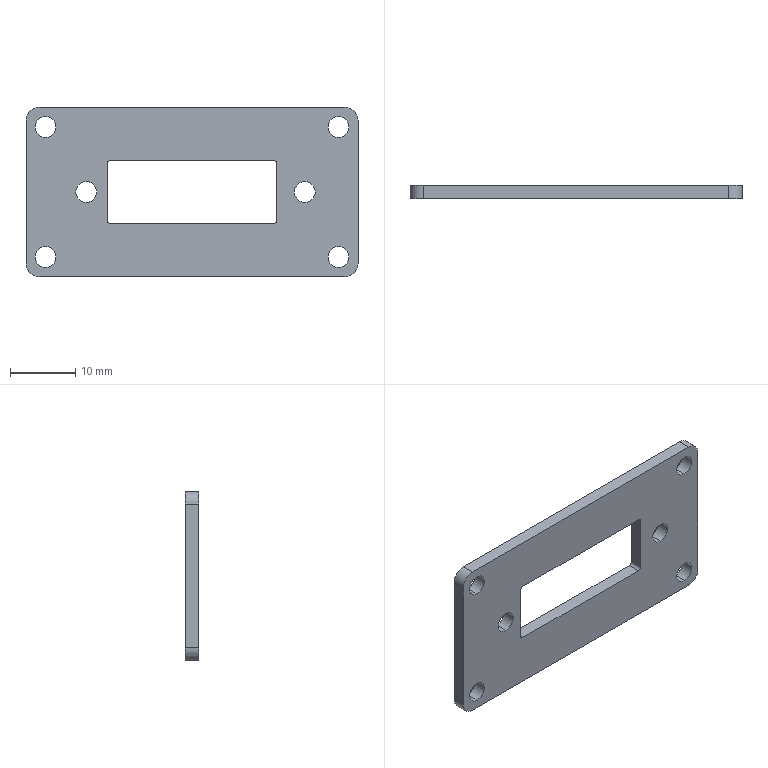Part | SolidWorks | features Cut 1, Extrusion 1, Fillet 1 | 1 solid | 30 faces | box 51 x 2 x 26 mm | volume 2048 mm3 | cylinder 20 | plane 10 | commonest cylinder face diameters 3.2 x12 1 x4 4 x4
STEP:
#1=CARTESIAN_POINT('',(17.311,2.,1.6));
#2=VERTEX_POINT('',#1);
#3=CARTESIAN_POINT('',(17.311,2.,-1.6));
#4=VERTEX_POINT('',#3);
#5=CARTESIAN_POINT('',(17.311,2.,0.));
#6=DIRECTION('',(0.,-1.,0.));
#7=DIRECTION('',(0.,0.,-1.));
#8=AXIS2_PLACEMENT_3D('',#5,#6,#7);
#9=CIRCLE('',#8,1.6);
#10=EDGE_CURVE('',#2,#4,#9,.T.);
#11=ORIENTED_EDGE('',*,*,#10,.F.);
#12=CARTESIAN_POINT('',(17.311,0.,1.6));
#13=VERTEX_POINT('',#12);
#14=CARTESIAN_POINT('',(17.311,2.,1.6));
#15=DIRECTION('',(0.,-1.,0.));
#16=VECTOR('',#15,1000.);
#17=LINE('',#14,#16);
#18=EDGE_CURVE('',#2,#13,#17,.T.);
#19=ORIENTED_EDGE('',*,*,#18,.T.);
#20=CARTESIAN_POINT('',(17.311,0.,-1.6));
#21=VERTEX_POINT('',#20);
#22=CARTESIAN_POINT('',(17.311,0.,0.));
#23=DIRECTION('',(0.,-1.,0.));
#24=DIRECTION('',(0.,0.,-1.));
#25=AXIS2_PLACEMENT_3D('',#22,#23,#24);
#26=CIRCLE('',#25,1.6);
#27=EDGE_CURVE('',#13,#21,#26,.T.);
#28=ORIENTED_EDGE('',*,*,#27,.T.);
#29=CARTESIAN_POINT('',(17.311,2.,-1.6));
#30=DIRECTION('',(0.,-1.,0.));
#31=VECTOR('',#30,1000.);
#32=LINE('',#29,#31);
#33=EDGE_CURVE('',#4,#21,#32,.T.);
#34=ORIENTED_EDGE('',*,*,#33,.F.);
#35=EDGE_LOOP('',(#11,#19,#28,#34));
#36=FACE_OUTER_BOUND('',#35,.T.);
#37=CARTESIAN_POINT('',(17.311,2.,0.));
#38=DIRECTION('',(0.,-1.,0.));
#39=DIRECTION('',(0.,0.,-1.));
#40=AXIS2_PLACEMENT_3D('',#37,#38,#39);
#41=CYLINDRICAL_SURFACE('',#40,1.6);
#42=ADVANCED_FACE('',(#36),#41,.F.);
#43=CARTESIAN_POINT('',(-16.25,2.,1.6));
#44=VERTEX_POINT('',#43);
#45=CARTESIAN_POINT('',(-16.25,2.,-1.6));
#46=VERTEX_POINT('',#45);
#47=CARTESIAN_POINT('',(-16.25,2.,0.));
#48=DIRECTION('',(0.,-1.,0.));
#49=DIRECTION('',(0.,0.,-1.));
#50=AXIS2_PLACEMENT_3D('',#47,#48,#49);
#51=CIRCLE('',#50,1.6);
#52=EDGE_CURVE('',#44,#46,#51,.T.);
#53=ORIENTED_EDGE('',*,*,#52,.F.);
#54=CARTESIAN_POINT('',(-16.25,0.,1.6));
#55=VERTEX_POINT('',#54);
#56=CARTESIAN_POINT('',(-16.25,2.,1.6));
#57=DIRECTION('',(0.,-1.,0.));
#58=VECTOR('',#57,1000.);
#59=LINE('',#56,#58);
#60=EDGE_CURVE('',#44,#55,#59,.T.);
#61=ORIENTED_EDGE('',*,*,#60,.T.);
#62=CARTESIAN_POINT('',(-16.25,0.,-1.6));
#63=VERTEX_POINT('',#62);
#64=CARTESIAN_POINT('',(-16.25,0.,0.));
#65=DIRECTION('',(0.,-1.,0.));
#66=DIRECTION('',(0.,0.,-1.));
#67=AXIS2_PLACEMENT_3D('',#64,#65,#66);
#68=CIRCLE('',#67,1.6);
#69=EDGE_CURVE('',#55,#63,#68,.T.);
#70=ORIENTED_EDGE('',*,*,#69,.T.);
#71=CARTESIAN_POINT('',(-16.25,2.,-1.6));
#72=DIRECTION('',(0.,-1.,0.));
#73=VECTOR('',#72,1000.);
#74=LINE('',#71,#73);
#75=EDGE_CURVE('',#46,#63,#74,.T.);
#76=ORIENTED_EDGE('',*,*,#75,.F.);
#77=EDGE_LOOP('',(#53,#61,#70,#76));
#78=FACE_OUTER_BOUND('',#77,.T.);
#79=CARTESIAN_POINT('',(-16.25,2.,0.));
#80=DIRECTION('',(0.,-1.,0.));
#81=DIRECTION('',(0.,0.,-1.));
#82=AXIS2_PLACEMENT_3D('',#79,#80,#81);
#83=CYLINDRICAL_SURFACE('',#82,1.6);
#84=ADVANCED_FACE('',(#78),#83,.F.);
#85=CARTESIAN_POINT('',(-22.5,2.,8.4));
#86=VERTEX_POINT('',#85);
#87=CARTESIAN_POINT('',(-22.5,2.,11.6));
#88=VERTEX_POINT('',#87);
#89=CARTESIAN_POINT('',(-22.5,2.,10.));
#90=DIRECTION('',(0.,1.,0.));
#91=DIRECTION('',(0.,0.,1.));
#92=AXIS2_PLACEMENT_3D('',#89,#90,#91);
#93=CIRCLE('',#92,1.6);
#94=EDGE_CURVE('',#86,#88,#93,.T.);
#95=ORIENTED_EDGE('',*,*,#94,.T.);
#96=CARTESIAN_POINT('',(-22.5,0.,11.6));
#97=VERTEX_POINT('',#96);
#98=CARTESIAN_POINT('',(-22.5,2.,11.6));
#99=DIRECTION('',(0.,-1.,0.));
#100=VECTOR('',#99,1000.);
#101=LINE('',#98,#100);
#102=EDGE_CURVE('',#88,#97,#101,.T.);
#103=ORIENTED_EDGE('',*,*,#102,.T.);
#104=CARTESIAN_POINT('',(-22.5,0.,8.4));
#105=VERTEX_POINT('',#104);
#106=CARTESIAN_POINT('',(-22.5,0.,10.));
#107=DIRECTION('',(0.,1.,0.));
#108=DIRECTION('',(0.,0.,1.));
#109=AXIS2_PLACEMENT_3D('',#106,#107,#108);
#110=CIRCLE('',#109,1.6);
#111=EDGE_CURVE('',#105,#97,#110,.T.);
#112=ORIENTED_EDGE('',*,*,#111,.F.);
#113=CARTESIAN_POINT('',(-22.5,2.,8.4));
#114=DIRECTION('',(0.,-1.,0.));
#115=VECTOR('',#114,1000.);
#116=LINE('',#113,#115);
#117=EDGE_CURVE('',#86,#105,#116,.T.);
#118=ORIENTED_EDGE('',*,*,#117,.F.);
#119=EDGE_LOOP('',(#95,#103,#112,#118));
#120=FACE_OUTER_BOUND('',#119,.T.);
#121=CARTESIAN_POINT('',(-22.5,2.,10.));
#122=DIRECTION('',(0.,-1.,0.));
#123=DIRECTION('',(0.,0.,-1.));
#124=AXIS2_PLACEMENT_3D('',#121,#122,#123);
#125=CYLINDRICAL_SURFACE('',#124,1.6);
#126=ADVANCED_FACE('',(#120),#125,.F.);
#127=CARTESIAN_POINT('',(22.5,2.,8.4));
#128=VERTEX_POINT('',#127);
#129=CARTESIAN_POINT('',(22.5,2.,11.6));
#130=VERTEX_POINT('',#129);
#131=CARTESIAN_POINT('',(22.5,2.,10.));
#132=DIRECTION('',(0.,1.,0.));
#133=DIRECTION('',(0.,0.,1.));
#134=AXIS2_PLACEMENT_3D('',#131,#132,#133);
#135=CIRCLE('',#134,1.6);
#136=EDGE_CURVE('',#128,#130,#135,.T.);
#137=ORIENTED_EDGE('',*,*,#136,.T.);
#138=CARTESIAN_POINT('',(22.5,0.,11.6));
#139=VERTEX_POINT('',#138);
#140=CARTESIAN_POINT('',(22.5,2.,11.6));
#141=DIRECTION('',(0.,-1.,0.));
#142=VECTOR('',#141,1000.);
#143=LINE('',#140,#142);
#144=EDGE_CURVE('',#130,#139,#143,.T.);
#145=ORIENTED_EDGE('',*,*,#144,.T.);
#146=CARTESIAN_POINT('',(22.5,0.,8.4));
#147=VERTEX_POINT('',#146);
#148=CARTESIAN_POINT('',(22.5,0.,10.));
#149=DIRECTION('',(0.,1.,0.));
#150=DIRECTION('',(0.,0.,1.));
#151=AXIS2_PLACEMENT_3D('',#148,#149,#150);
#152=CIRCLE('',#151,1.6);
#153=EDGE_CURVE('',#147,#139,#152,.T.);
#154=ORIENTED_EDGE('',*,*,#153,.F.);
#155=CARTESIAN_POINT('',(22.5,2.,8.4));
#156=DIRECTION('',(0.,-1.,0.));
#157=VECTOR('',#156,1000.);
#158=LINE('',#155,#157);
#159=EDGE_CURVE('',#128,#147,#158,.T.);
#160=ORIENTED_EDGE('',*,*,#159,.F.);
#161=EDGE_LOOP('',(#137,#145,#154,#160));
#162=FACE_OUTER_BOUND('',#161,.T.);
#163=CARTESIAN_POINT('',(22.5,2.,10.));
#164=DIRECTION('',(0.,-1.,0.));
#165=DIRECTION('',(0.,0.,-1.));
#166=AXIS2_PLACEMENT_3D('',#163,#164,#165);
#167=CYLINDRICAL_SURFACE('',#166,1.6);
#168=ADVANCED_FACE('',(#162),#167,.F.);
#169=CARTESIAN_POINT('',(22.5,2.,-11.6));
#170=VERTEX_POINT('',#169);
#171=CARTESIAN_POINT('',(22.5,2.,-8.4));
#172=VERTEX_POINT('',#171);
#173=CARTESIAN_POINT('',(22.5,2.,-10.));
#174=DIRECTION('',(0.,1.,0.));
#175=DIRECTION('',(0.,0.,1.));
#176=AXIS2_PLACEMENT_3D('',#173,#174,#175);
#177=CIRCLE('',#176,1.6);
#178=EDGE_CURVE('',#170,#172,#177,.T.);
#179=ORIENTED_EDGE('',*,*,#178,.T.);
#180=CARTESIAN_POINT('',(22.5,0.,-8.4));
#181=VERTEX_POINT('',#180);
#182=CARTESIAN_POINT('',(22.5,2.,-8.4));
#183=DIRECTION('',(0.,-1.,0.));
#184=VECTOR('',#183,1000.);
#185=LINE('',#182,#184);
#186=EDGE_CURVE('',#172,#181,#185,.T.);
#187=ORIENTED_EDGE('',*,*,#186,.T.);
#188=CARTESIAN_POINT('',(22.5,0.,-11.6));
#189=VERTEX_POINT('',#188);
#190=CARTESIAN_POINT('',(22.5,0.,-10.));
#191=DIRECTION('',(0.,1.,0.));
#192=DIRECTION('',(0.,0.,1.));
#193=AXIS2_PLACEMENT_3D('',#190,#191,#192);
#194=CIRCLE('',#193,1.6);
#195=EDGE_CURVE('',#189,#181,#194,.T.);
#196=ORIENTED_EDGE('',*,*,#195,.F.);
#197=CARTESIAN_POINT('',(22.5,2.,-11.6));
#198=DIRECTION('',(0.,-1.,0.));
#199=VECTOR('',#198,1000.);
#200=LINE('',#197,#199);
#201=EDGE_CURVE('',#170,#189,#200,.T.);
#202=ORIENTED_EDGE('',*,*,#201,.F.);
#203=EDGE_LOOP('',(#179,#187,#196,#202));
#204=FACE_OUTER_BOUND('',#203,.T.);
#205=CARTESIAN_POINT('',(22.5,2.,-10.));
#206=DIRECTION('',(0.,-1.,0.));
#207=DIRECTION('',(0.,0.,-1.));
#208=AXIS2_PLACEMENT_3D('',#205,#206,#207);
#209=CYLINDRICAL_SURFACE('',#208,1.6);
#210=ADVANCED_FACE('',(#204),#209,.F.);
#211=CARTESIAN_POINT('',(-22.5,2.,-11.6));
#212=VERTEX_POINT('',#211);
#213=CARTESIAN_POINT('',(-22.5,2.,-8.4));
#214=VERTEX_POINT('',#213);
#215=CARTESIAN_POINT('',(-22.5,2.,-10.));
#216=DIRECTION('',(0.,1.,0.));
#217=DIRECTION('',(0.,0.,1.));
#218=AXIS2_PLACEMENT_3D('',#215,#216,#217);
#219=CIRCLE('',#218,1.6);
#220=EDGE_CURVE('',#212,#214,#219,.T.);
#221=ORIENTED_EDGE('',*,*,#220,.T.);
#222=CARTESIAN_POINT('',(-22.5,0.,-8.4));
#223=VERTEX_POINT('',#222);
#224=CARTESIAN_POINT('',(-22.5,2.,-8.4));
#225=DIRECTION('',(0.,-1.,0.));
#226=VECTOR('',#225,1000.);
#227=LINE('',#224,#226);
#228=EDGE_CURVE('',#214,#223,#227,.T.);
#229=ORIENTED_EDGE('',*,*,#228,.T.);
#230=CARTESIAN_POINT('',(-22.5,0.,-11.6));
#231=VERTEX_POINT('',#230);
#232=CARTESIAN_POINT('',(-22.5,0.,-10.));
#233=DIRECTION('',(0.,1.,0.));
#234=DIRECTION('',(0.,0.,1.));
#235=AXIS2_PLACEMENT_3D('',#232,#233,#234);
#236=CIRCLE('',#235,1.6);
#237=EDGE_CURVE('',#231,#223,#236,.T.);
#238=ORIENTED_EDGE('',*,*,#237,.F.);
#239=CARTESIAN_POINT('',(-22.5,2.,-11.6));
#240=DIRECTION('',(0.,-1.,0.));
#241=VECTOR('',#240,1000.);
#242=LINE('',#239,#241);
#243=EDGE_CURVE('',#212,#231,#242,.T.);
#244=ORIENTED_EDGE('',*,*,#243,.F.);
#245=EDGE_LOOP('',(#221,#229,#238,#244));
#246=FACE_OUTER_BOUND('',#245,.T.);
#247=CARTESIAN_POINT('',(-22.5,2.,-10.));
#248=DIRECTION('',(0.,-1.,0.));
#249=DIRECTION('',(0.,0.,-1.));
#250=AXIS2_PLACEMENT_3D('',#247,#248,#249);
#251=CYLINDRICAL_SURFACE('',#250,1.6);
#252=ADVANCED_FACE('',(#246),#251,.F.);
#253=CARTESIAN_POINT('',(17.311,2.,0.));
#254=DIRECTION('',(0.,-1.,0.));
#255=DIRECTION('',(0.,0.,-1.));
#256=AXIS2_PLACEMENT_3D('',#253,#254,#255);
#257=CIRCLE('',#256,1.6);
#258=EDGE_CURVE('',#4,#2,#257,.T.);
#259=ORIENTED_EDGE('',*,*,#258,.T.);
#260=ORIENTED_EDGE('',*,*,#10,.T.);
#261=EDGE_LOOP('',(#259,#260));
#262=FACE_BOUND('',#261,.T.);
#263=CARTESIAN_POINT('',(-16.25,2.,0.));
#264=DIRECTION('',(0.,-1.,0.));
#265=DIRECTION('',(0.,0.,-1.));
#266=AXIS2_PLACEMENT_3D('',#263,#264,#265);
#267=CIRCLE('',#266,1.6);
#268=EDGE_CURVE('',#46,#44,#267,.T.);
#269=ORIENTED_EDGE('',*,*,#268,.T.);
#270=ORIENTED_EDGE('',*,*,#52,.T.);
#271=EDGE_LOOP('',(#269,#270));
#272=FACE_BOUND('',#271,.T.);
#273=CARTESIAN_POINT('',(-13.05,2.,4.3));
#274=VERTEX_POINT('',#273);
#275=CARTESIAN_POINT('',(-13.05,2.,-4.3));
#276=VERTEX_POINT('',#275);
#277=CARTESIAN_POINT('',(-13.05,2.,-4.8));
#278=DIRECTION('',(0.,0.,-1.));
#279=VECTOR('',#278,1000.);
#280=LINE('',#277,#279);
#281=EDGE_CURVE('',#274,#276,#280,.T.);
#282=ORIENTED_EDGE('',*,*,#281,.T.);
#283=CARTESIAN_POINT('',(-12.55,2.,-4.8));
#284=VERTEX_POINT('',#283);
#285=CARTESIAN_POINT('',(-12.55,2.,-4.3));
#286=DIRECTION('',(0.,-1.,0.));
#287=DIRECTION('',(0.,0.,-1.));
#288=AXIS2_PLACEMENT_3D('',#285,#286,#287);
#289=CIRCLE('',#288,0.5);
#290=EDGE_CURVE('',#276,#284,#289,.T.);
#291=ORIENTED_EDGE('',*,*,#290,.T.);
#292=CARTESIAN_POINT('',(12.55,2.,-4.8));
#293=VERTEX_POINT('',#292);
#294=CARTESIAN_POINT('',(-13.05,2.,-4.8));
#295=DIRECTION('',(1.,0.,0.));
#296=VECTOR('',#295,1000.);
#297=LINE('',#294,#296);
#298=EDGE_CURVE('',#284,#293,#297,.T.);
#299=ORIENTED_EDGE('',*,*,#298,.T.);
#300=CARTESIAN_POINT('',(13.05,2.,-4.3));
#301=VERTEX_POINT('',#300);
#302=CARTESIAN_POINT('',(12.55,2.,-4.3));
#303=DIRECTION('',(0.,-1.,0.));
#304=DIRECTION('',(0.,0.,-1.));
#305=AXIS2_PLACEMENT_3D('',#302,#303,#304);
#306=CIRCLE('',#305,0.5);
#307=EDGE_CURVE('',#293,#301,#306,.T.);
#308=ORIENTED_EDGE('',*,*,#307,.T.);
#309=CARTESIAN_POINT('',(13.05,2.,4.3));
#310=VERTEX_POINT('',#309);
#311=CARTESIAN_POINT('',(13.05,2.,-4.8));
#312=DIRECTION('',(0.,0.,1.));
#313=VECTOR('',#312,1000.);
#314=LINE('',#311,#313);
#315=EDGE_CURVE('',#301,#310,#314,.T.);
#316=ORIENTED_EDGE('',*,*,#315,.T.);
#317=CARTESIAN_POINT('',(12.55,2.,4.8));
#318=VERTEX_POINT('',#317);
#319=CARTESIAN_POINT('',(12.55,2.,4.3));
#320=DIRECTION('',(0.,-1.,0.));
#321=DIRECTION('',(0.,0.,-1.));
#322=AXIS2_PLACEMENT_3D('',#319,#320,#321);
#323=CIRCLE('',#322,0.5);
#324=EDGE_CURVE('',#310,#318,#323,.T.);
#325=ORIENTED_EDGE('',*,*,#324,.T.);
#326=CARTESIAN_POINT('',(-12.55,2.,4.8));
#327=VERTEX_POINT('',#326);
#328=CARTESIAN_POINT('',(-13.05,2.,4.8));
#329=DIRECTION('',(-1.,0.,0.));
#330=VECTOR('',#329,1000.);
#331=LINE('',#328,#330);
#332=EDGE_CURVE('',#318,#327,#331,.T.);
#333=ORIENTED_EDGE('',*,*,#332,.T.);
#334=CARTESIAN_POINT('',(-12.55,2.,4.3));
#335=DIRECTION('',(0.,-1.,0.));
#336=DIRECTION('',(0.,0.,-1.));
#337=AXIS2_PLACEMENT_3D('',#334,#335,#336);
#338=CIRCLE('',#337,0.5);
#339=EDGE_CURVE('',#327,#274,#338,.T.);
#340=ORIENTED_EDGE('',*,*,#339,.T.);
#341=EDGE_LOOP('',(#282,#291,#299,#308,#316,#325,#333,#340));
#342=FACE_BOUND('',#341,.T.);
#343=CARTESIAN_POINT('',(25.5,2.,-11.));
#344=VERTEX_POINT('',#343);
#345=CARTESIAN_POINT('',(23.5,2.,-13.));
#346=VERTEX_POINT('',#345);
#347=CARTESIAN_POINT('',(23.5,2.,-11.));
#348=DIRECTION('',(0.,1.,0.));
#349=DIRECTION('',(0.,0.,-1.));
#350=AXIS2_PLACEMENT_3D('',#347,#348,#349);
#351=CIRCLE('',#350,2.);
#352=EDGE_CURVE('',#344,#346,#351,.T.);
#353=ORIENTED_EDGE('',*,*,#352,.T.);
#354=CARTESIAN_POINT('',(-23.5,2.,-13.));
#355=VERTEX_POINT('',#354);
#356=CARTESIAN_POINT('',(-23.5,2.,-13.));
#357=DIRECTION('',(-1.,0.,0.));
#358=VECTOR('',#357,1000.);
#359=LINE('',#356,#358);
#360=EDGE_CURVE('',#346,#355,#359,.T.);
#361=ORIENTED_EDGE('',*,*,#360,.T.);
#362=CARTESIAN_POINT('',(-25.5,2.,-11.));
#363=VERTEX_POINT('',#362);
#364=CARTESIAN_POINT('',(-23.5,2.,-11.));
#365=DIRECTION('',(0.,1.,0.));
#366=DIRECTION('',(0.,0.,-1.));
#367=AXIS2_PLACEMENT_3D('',#364,#365,#366);
#368=CIRCLE('',#367,2.);
#369=EDGE_CURVE('',#355,#363,#368,.T.);
#370=ORIENTED_EDGE('',*,*,#369,.T.);
#371=CARTESIAN_POINT('',(-25.5,2.,11.));
#372=VERTEX_POINT('',#371);
#373=CARTESIAN_POINT('',(-25.5,2.,11.));
#374=DIRECTION('',(0.,0.,1.));
#375=VECTOR('',#374,1000.);
#376=LINE('',#373,#375);
#377=EDGE_CURVE('',#363,#372,#376,.T.);
#378=ORIENTED_EDGE('',*,*,#377,.T.);
#379=CARTESIAN_POINT('',(-23.5,2.,13.));
#380=VERTEX_POINT('',#379);
#381=CARTESIAN_POINT('',(-23.5,2.,11.));
#382=DIRECTION('',(0.,1.,0.));
#383=DIRECTION('',(0.,0.,-1.));
#384=AXIS2_PLACEMENT_3D('',#381,#382,#383);
#385=CIRCLE('',#384,2.);
#386=EDGE_CURVE('',#372,#380,#385,.T.);
#387=ORIENTED_EDGE('',*,*,#386,.T.);
#388=CARTESIAN_POINT('',(23.5,2.,13.));
#389=VERTEX_POINT('',#388);
#390=CARTESIAN_POINT('',(-23.5,2.,13.));
#391=DIRECTION('',(1.,0.,0.));
#392=VECTOR('',#391,1000.);
#393=LINE('',#390,#392);
#394=EDGE_CURVE('',#380,#389,#393,.T.);
#395=ORIENTED_EDGE('',*,*,#394,.T.);
#396=CARTESIAN_POINT('',(25.5,2.,11.));
#397=VERTEX_POINT('',#396);
#398=CARTESIAN_POINT('',(23.5,2.,11.));
#399=DIRECTION('',(0.,1.,0.));
#400=DIRECTION('',(0.,0.,1.));
#401=AXIS2_PLACEMENT_3D('',#398,#399,#400);
#402=CIRCLE('',#401,2.);
#403=EDGE_CURVE('',#389,#397,#402,.T.);
#404=ORIENTED_EDGE('',*,*,#403,.T.);
#405=CARTESIAN_POINT('',(25.5,2.,11.));
#406=DIRECTION('',(0.,0.,-1.));
#407=VECTOR('',#406,1000.);
#408=LINE('',#405,#407);
#409=EDGE_CURVE('',#397,#344,#408,.T.);
#410=ORIENTED_EDGE('',*,*,#409,.T.);
#411=EDGE_LOOP('',(#353,#361,#370,#378,#387,#395,#404,#410));
#412=FACE_OUTER_BOUND('',#411,.T.);
#413=ORIENTED_EDGE('',*,*,#220,.F.);
#414=CARTESIAN_POINT('',(-22.5,2.,-10.));
#415=DIRECTION('',(0.,1.,0.));
#416=DIRECTION('',(0.,0.,1.));
#417=AXIS2_PLACEMENT_3D('',#414,#415,#416);
#418=CIRCLE('',#417,1.6);
#419=EDGE_CURVE('',#214,#212,#418,.T.);
#420=ORIENTED_EDGE('',*,*,#419,.F.);
#421=EDGE_LOOP('',(#413,#420));
#422=FACE_BOUND('',#421,.T.);
#423=ORIENTED_EDGE('',*,*,#178,.F.);
#424=CARTESIAN_POINT('',(22.5,2.,-10.));
#425=DIRECTION('',(0.,1.,0.));
#426=DIRECTION('',(0.,0.,1.));
#427=AXIS2_PLACEMENT_3D('',#424,#425,#426);
#428=CIRCLE('',#427,1.6);
#429=EDGE_CURVE('',#172,#170,#428,.T.);
#430=ORIENTED_EDGE('',*,*,#429,.F.);
#431=EDGE_LOOP('',(#423,#430));
#432=FACE_BOUND('',#431,.T.);
#433=ORIENTED_EDGE('',*,*,#136,.F.);
#434=CARTESIAN_POINT('',(22.5,2.,10.));
#435=DIRECTION('',(0.,1.,0.));
#436=DIRECTION('',(0.,0.,1.));
#437=AXIS2_PLACEMENT_3D('',#434,#435,#436);
#438=CIRCLE('',#437,1.6);
#439=EDGE_CURVE('',#130,#128,#438,.T.);
#440=ORIENTED_EDGE('',*,*,#439,.F.);
#441=EDGE_LOOP('',(#433,#440));
#442=FACE_BOUND('',#441,.T.);
#443=ORIENTED_EDGE('',*,*,#94,.F.);
#444=CARTESIAN_POINT('',(-22.5,2.,10.));
#445=DIRECTION('',(0.,1.,0.));
#446=DIRECTION('',(0.,0.,1.));
#447=AXIS2_PLACEMENT_3D('',#444,#445,#446);
#448=CIRCLE('',#447,1.6);
#449=EDGE_CURVE('',#88,#86,#448,.T.);
#450=ORIENTED_EDGE('',*,*,#449,.F.);
#451=EDGE_LOOP('',(#443,#450));
#452=FACE_BOUND('',#451,.T.);
#453=CARTESIAN_POINT('',(23.5,2.,-11.));
#454=DIRECTION('',(0.,-1.,0.));
#455=DIRECTION('',(0.,0.,-1.));
#456=AXIS2_PLACEMENT_3D('',#453,#454,#455);
#457=PLANE('',#456);
#458=ADVANCED_FACE('',(#262,#272,#342,#412,#422,#432,#442,#452),#457,.F.);
#459=CARTESIAN_POINT('',(17.311,0.,0.));
#460=DIRECTION('',(0.,-1.,0.));
#461=DIRECTION('',(0.,0.,-1.));
#462=AXIS2_PLACEMENT_3D('',#459,#460,#461);
#463=CIRCLE('',#462,1.6);
#464=EDGE_CURVE('',#21,#13,#463,.T.);
#465=ORIENTED_EDGE('',*,*,#464,.F.);
#466=ORIENTED_EDGE('',*,*,#27,.F.);
#467=EDGE_LOOP('',(#465,#466));
#468=FACE_BOUND('',#467,.T.);
#469=CARTESIAN_POINT('',(-16.25,0.,0.));
#470=DIRECTION('',(0.,-1.,0.));
#471=DIRECTION('',(0.,0.,-1.));
#472=AXIS2_PLACEMENT_3D('',#469,#470,#471);
#473=CIRCLE('',#472,1.6);
#474=EDGE_CURVE('',#63,#55,#473,.T.);
#475=ORIENTED_EDGE('',*,*,#474,.F.);
#476=ORIENTED_EDGE('',*,*,#69,.F.);
#477=EDGE_LOOP('',(#475,#476));
#478=FACE_BOUND('',#477,.T.);
#479=CARTESIAN_POINT('',(13.05,0.,-4.3));
#480=VERTEX_POINT('',#479);
#481=CARTESIAN_POINT('',(13.05,0.,4.3));
#482=VERTEX_POINT('',#481);
#483=CARTESIAN_POINT('',(13.05,0.,-4.8));
#484=DIRECTION('',(0.,0.,1.));
#485=VECTOR('',#484,1000.);
#486=LINE('',#483,#485);
#487=EDGE_CURVE('',#480,#482,#486,.T.);
#488=ORIENTED_EDGE('',*,*,#487,.F.);
#489=CARTESIAN_POINT('',(12.55,0.,-4.8));
#490=VERTEX_POINT('',#489);
#491=CARTESIAN_POINT('',(12.55,0.,-4.3));
#492=DIRECTION('',(0.,1.,0.));
#493=DIRECTION('',(0.,0.,-1.));
#494=AXIS2_PLACEMENT_3D('',#491,#492,#493);
#495=CIRCLE('',#494,0.5);
#496=EDGE_CURVE('',#480,#490,#495,.T.);
#497=ORIENTED_EDGE('',*,*,#496,.T.);
#498=CARTESIAN_POINT('',(-12.55,0.,-4.8));
#499=VERTEX_POINT('',#498);
#500=CARTESIAN_POINT('',(-13.05,0.,-4.8));
#501=DIRECTION('',(1.,0.,0.));
#502=VECTOR('',#501,1000.);
#503=LINE('',#500,#502);
#504=EDGE_CURVE('',#499,#490,#503,.T.);
#505=ORIENTED_EDGE('',*,*,#504,.F.);
#506=CARTESIAN_POINT('',(-13.05,0.,-4.3));
#507=VERTEX_POINT('',#506);
#508=CARTESIAN_POINT('',(-12.55,0.,-4.3));
#509=DIRECTION('',(0.,1.,0.));
#510=DIRECTION('',(0.,0.,-1.));
#511=AXIS2_PLACEMENT_3D('',#508,#509,#510);
#512=CIRCLE('',#511,0.5);
#513=EDGE_CURVE('',#499,#507,#512,.T.);
#514=ORIENTED_EDGE('',*,*,#513,.T.);
#515=CARTESIAN_POINT('',(-13.05,0.,4.3));
#516=VERTEX_POINT('',#515);
#517=CARTESIAN_POINT('',(-13.05,0.,-4.8));
#518=DIRECTION('',(0.,0.,-1.));
#519=VECTOR('',#518,1000.);
#520=LINE('',#517,#519);
#521=EDGE_CURVE('',#516,#507,#520,.T.);
#522=ORIENTED_EDGE('',*,*,#521,.F.);
#523=CARTESIAN_POINT('',(-12.55,0.,4.8));
#524=VERTEX_POINT('',#523);
#525=CARTESIAN_POINT('',(-12.55,0.,4.3));
#526=DIRECTION('',(0.,1.,0.));
#527=DIRECTION('',(0.,0.,-1.));
#528=AXIS2_PLACEMENT_3D('',#525,#526,#527);
#529=CIRCLE('',#528,0.5);
#530=EDGE_CURVE('',#516,#524,#529,.T.);
#531=ORIENTED_EDGE('',*,*,#530,.T.);
#532=CARTESIAN_POINT('',(12.55,0.,4.8));
#533=VERTEX_POINT('',#532);
#534=CARTESIAN_POINT('',(-13.05,0.,4.8));
#535=DIRECTION('',(-1.,0.,0.));
#536=VECTOR('',#535,1000.);
#537=LINE('',#534,#536);
#538=EDGE_CURVE('',#533,#524,#537,.T.);
#539=ORIENTED_EDGE('',*,*,#538,.F.);
#540=CARTESIAN_POINT('',(12.55,0.,4.3));
#541=DIRECTION('',(0.,1.,0.));
#542=DIRECTION('',(0.,0.,-1.));
#543=AXIS2_PLACEMENT_3D('',#540,#541,#542);
#544=CIRCLE('',#543,0.5);
#545=EDGE_CURVE('',#533,#482,#544,.T.);
#546=ORIENTED_EDGE('',*,*,#545,.T.);
#547=EDGE_LOOP('',(#488,#497,#505,#514,#522,#531,#539,#546));
#548=FACE_BOUND('',#547,.T.);
#549=ORIENTED_EDGE('',*,*,#153,.T.);
#550=CARTESIAN_POINT('',(22.5,0.,10.));
#551=DIRECTION('',(0.,1.,0.));
#552=DIRECTION('',(0.,0.,1.));
#553=AXIS2_PLACEMENT_3D('',#550,#551,#552);
#554=CIRCLE('',#553,1.6);
#555=EDGE_CURVE('',#139,#147,#554,.T.);
#556=ORIENTED_EDGE('',*,*,#555,.T.);
#557=EDGE_LOOP('',(#549,#556));
#558=FACE_BOUND('',#557,.T.);
#559=ORIENTED_EDGE('',*,*,#237,.T.);
#560=CARTESIAN_POINT('',(-22.5,0.,-10.));
#561=DIRECTION('',(0.,1.,0.));
#562=DIRECTION('',(0.,0.,1.));
#563=AXIS2_PLACEMENT_3D('',#560,#561,#562);
#564=CIRCLE('',#563,1.6);
#565=EDGE_CURVE('',#223,#231,#564,.T.);
#566=ORIENTED_EDGE('',*,*,#565,.T.);
#567=EDGE_LOOP('',(#559,#566));
#568=FACE_BOUND('',#567,.T.);
#569=CARTESIAN_POINT('',(25.5,0.,-11.));
#570=VERTEX_POINT('',#569);
#571=CARTESIAN_POINT('',(23.5,0.,-13.));
#572=VERTEX_POINT('',#571);
#573=CARTESIAN_POINT('',(23.5,0.,-11.));
#574=DIRECTION('',(0.,1.,0.));
#575=DIRECTION('',(0.,0.,-1.));
#576=AXIS2_PLACEMENT_3D('',#573,#574,#575);
#577=CIRCLE('',#576,2.);
#578=EDGE_CURVE('',#570,#572,#577,.T.);
#579=ORIENTED_EDGE('',*,*,#578,.F.);
#580=CARTESIAN_POINT('',(25.5,0.,11.));
#581=VERTEX_POINT('',#580);
#582=CARTESIAN_POINT('',(25.5,0.,11.));
#583=DIRECTION('',(0.,0.,-1.));
#584=VECTOR('',#583,1000.);
#585=LINE('',#582,#584);
#586=EDGE_CURVE('',#581,#570,#585,.T.);
#587=ORIENTED_EDGE('',*,*,#586,.F.);
#588=CARTESIAN_POINT('',(23.5,0.,13.));
#589=VERTEX_POINT('',#588);
#590=CARTESIAN_POINT('',(23.5,0.,11.));
#591=DIRECTION('',(0.,1.,0.));
#592=DIRECTION('',(0.,0.,1.));
#593=AXIS2_PLACEMENT_3D('',#590,#591,#592);
#594=CIRCLE('',#593,2.);
#595=EDGE_CURVE('',#589,#581,#594,.T.);
#596=ORIENTED_EDGE('',*,*,#595,.F.);
#597=CARTESIAN_POINT('',(-23.5,0.,13.));
#598=VERTEX_POINT('',#597);
#599=CARTESIAN_POINT('',(-23.5,0.,13.));
#600=DIRECTION('',(1.,0.,0.));
#601=VECTOR('',#600,1000.);
#602=LINE('',#599,#601);
#603=EDGE_CURVE('',#598,#589,#602,.T.);
#604=ORIENTED_EDGE('',*,*,#603,.F.);
#605=CARTESIAN_POINT('',(-25.5,0.,11.));
#606=VERTEX_POINT('',#605);
#607=CARTESIAN_POINT('',(-23.5,0.,11.));
#608=DIRECTION('',(0.,1.,0.));
#609=DIRECTION('',(0.,0.,-1.));
#610=AXIS2_PLACEMENT_3D('',#607,#608,#609);
#611=CIRCLE('',#610,2.);
#612=EDGE_CURVE('',#606,#598,#611,.T.);
#613=ORIENTED_EDGE('',*,*,#612,.F.);
#614=CARTESIAN_POINT('',(-25.5,0.,-11.));
#615=VERTEX_POINT('',#614);
#616=CARTESIAN_POINT('',(-25.5,0.,11.));
#617=DIRECTION('',(0.,0.,1.));
#618=VECTOR('',#617,1000.);
#619=LINE('',#616,#618);
#620=EDGE_CURVE('',#615,#606,#619,.T.);
#621=ORIENTED_EDGE('',*,*,#620,.F.);
#622=CARTESIAN_POINT('',(-23.5,0.,-13.));
#623=VERTEX_POINT('',#622);
#624=CARTESIAN_POINT('',(-23.5,0.,-11.));
#625=DIRECTION('',(0.,1.,0.));
#626=DIRECTION('',(0.,0.,-1.));
#627=AXIS2_PLACEMENT_3D('',#624,#625,#626);
#628=CIRCLE('',#627,2.);
#629=EDGE_CURVE('',#623,#615,#628,.T.);
#630=ORIENTED_EDGE('',*,*,#629,.F.);
#631=CARTESIAN_POINT('',(-23.5,0.,-13.));
#632=DIRECTION('',(-1.,0.,0.));
#633=VECTOR('',#632,1000.);
#634=LINE('',#631,#633);
#635=EDGE_CURVE('',#572,#623,#634,.T.);
#636=ORIENTED_EDGE('',*,*,#635,.F.);
#637=EDGE_LOOP('',(#579,#587,#596,#604,#613,#621,#630,#636));
#638=FACE_OUTER_BOUND('',#637,.T.);
#639=ORIENTED_EDGE('',*,*,#195,.T.);
#640=CARTESIAN_POINT('',(22.5,0.,-10.));
#641=DIRECTION('',(0.,1.,0.));
#642=DIRECTION('',(0.,0.,1.));
#643=AXIS2_PLACEMENT_3D('',#640,#641,#642);
#644=CIRCLE('',#643,1.6);
#645=EDGE_CURVE('',#181,#189,#644,.T.);
#646=ORIENTED_EDGE('',*,*,#645,.T.);
#647=EDGE_LOOP('',(#639,#646));
#648=FACE_BOUND('',#647,.T.);
#649=ORIENTED_EDGE('',*,*,#111,.T.);
#650=CARTESIAN_POINT('',(-22.5,0.,10.));
#651=DIRECTION('',(0.,1.,0.));
#652=DIRECTION('',(0.,0.,1.));
#653=AXIS2_PLACEMENT_3D('',#650,#651,#652);
#654=CIRCLE('',#653,1.6);
#655=EDGE_CURVE('',#97,#105,#654,.T.);
#656=ORIENTED_EDGE('',*,*,#655,.T.);
#657=EDGE_LOOP('',(#649,#656));
#658=FACE_BOUND('',#657,.T.);
#659=CARTESIAN_POINT('',(23.5,0.,-11.));
#660=DIRECTION('',(0.,-1.,0.));
#661=DIRECTION('',(0.,0.,-1.));
#662=AXIS2_PLACEMENT_3D('',#659,#660,#661);
#663=PLANE('',#662);
#664=ADVANCED_FACE('',(#468,#478,#548,#558,#568,#638,#648,#658),#663,.T.);
#665=ORIENTED_EDGE('',*,*,#578,.T.);
#666=CARTESIAN_POINT('',(23.5,2.,-13.));
#667=DIRECTION('',(0.,-1.,0.));
#668=VECTOR('',#667,1000.);
#669=LINE('',#666,#668);
#670=EDGE_CURVE('',#346,#572,#669,.T.);
#671=ORIENTED_EDGE('',*,*,#670,.F.);
#672=ORIENTED_EDGE('',*,*,#352,.F.);
#673=CARTESIAN_POINT('',(25.5,2.,-11.));
#674=DIRECTION('',(0.,-1.,0.));
#675=VECTOR('',#674,1000.);
#676=LINE('',#673,#675);
#677=EDGE_CURVE('',#344,#570,#676,.T.);
#678=ORIENTED_EDGE('',*,*,#677,.T.);
#679=EDGE_LOOP('',(#665,#671,#672,#678));
#680=FACE_OUTER_BOUND('',#679,.T.);
#681=CARTESIAN_POINT('',(23.5,2.,-11.));
#682=DIRECTION('',(0.,-1.,0.));
#683=DIRECTION('',(0.,0.,-1.));
#684=AXIS2_PLACEMENT_3D('',#681,#682,#683);
#685=CYLINDRICAL_SURFACE('',#684,2.);
#686=ADVANCED_FACE('',(#680),#685,.T.);
#687=ORIENTED_EDGE('',*,*,#635,.T.);
#688=CARTESIAN_POINT('',(-23.5,2.,-13.));
#689=DIRECTION('',(0.,-1.,0.));
#690=VECTOR('',#689,1000.);
#691=LINE('',#688,#690);
#692=EDGE_CURVE('',#355,#623,#691,.T.);
#693=ORIENTED_EDGE('',*,*,#692,.F.);
#694=ORIENTED_EDGE('',*,*,#360,.F.);
#695=ORIENTED_EDGE('',*,*,#670,.T.);
#696=EDGE_LOOP('',(#687,#693,#694,#695));
#697=FACE_OUTER_BOUND('',#696,.T.);
#698=CARTESIAN_POINT('',(-23.5,2.,-13.));
#699=DIRECTION('',(0.,0.,1.));
#700=DIRECTION('',(1.,0.,0.));
#701=AXIS2_PLACEMENT_3D('',#698,#699,#700);
#702=PLANE('',#701);
#703=ADVANCED_FACE('',(#697),#702,.F.);
#704=ORIENTED_EDGE('',*,*,#629,.T.);
#705=CARTESIAN_POINT('',(-25.5,2.,-11.));
#706=DIRECTION('',(0.,-1.,0.));
#707=VECTOR('',#706,1000.);
#708=LINE('',#705,#707);
#709=EDGE_CURVE('',#363,#615,#708,.T.);
#710=ORIENTED_EDGE('',*,*,#709,.F.);
#711=ORIENTED_EDGE('',*,*,#369,.F.);
#712=ORIENTED_EDGE('',*,*,#692,.T.);
#713=EDGE_LOOP('',(#704,#710,#711,#712));
#714=FACE_OUTER_BOUND('',#713,.T.);
#715=CARTESIAN_POINT('',(-23.5,2.,-11.));
#716=DIRECTION('',(0.,-1.,0.));
#717=DIRECTION('',(0.,0.,-1.));
#718=AXIS2_PLACEMENT_3D('',#715,#716,#717);
#719=CYLINDRICAL_SURFACE('',#718,2.);
#720=ADVANCED_FACE('',(#714),#719,.T.);
#721=ORIENTED_EDGE('',*,*,#620,.T.);
#722=CARTESIAN_POINT('',(-25.5,2.,11.));
#723=DIRECTION('',(0.,-1.,0.));
#724=VECTOR('',#723,1000.);
#725=LINE('',#722,#724);
#726=EDGE_CURVE('',#372,#606,#725,.T.);
#727=ORIENTED_EDGE('',*,*,#726,.F.);
#728=ORIENTED_EDGE('',*,*,#377,.F.);
#729=ORIENTED_EDGE('',*,*,#709,.T.);
#730=EDGE_LOOP('',(#721,#727,#728,#729));
#731=FACE_OUTER_BOUND('',#730,.T.);
#732=CARTESIAN_POINT('',(-25.5,2.,11.));
#733=DIRECTION('',(1.,0.,0.));
#734=DIRECTION('',(0.,0.,-1.));
#735=AXIS2_PLACEMENT_3D('',#732,#733,#734);
#736=PLANE('',#735);
#737=ADVANCED_FACE('',(#731),#736,.F.);
#738=ORIENTED_EDGE('',*,*,#612,.T.);
#739=CARTESIAN_POINT('',(-23.5,2.,13.));
#740=DIRECTION('',(0.,-1.,0.));
#741=VECTOR('',#740,1000.);
#742=LINE('',#739,#741);
#743=EDGE_CURVE('',#380,#598,#742,.T.);
#744=ORIENTED_EDGE('',*,*,#743,.F.);
#745=ORIENTED_EDGE('',*,*,#386,.F.);
#746=ORIENTED_EDGE('',*,*,#726,.T.);
#747=EDGE_LOOP('',(#738,#744,#745,#746));
#748=FACE_OUTER_BOUND('',#747,.T.);
#749=CARTESIAN_POINT('',(-23.5,2.,11.));
#750=DIRECTION('',(0.,-1.,0.));
#751=DIRECTION('',(0.,0.,-1.));
#752=AXIS2_PLACEMENT_3D('',#749,#750,#751);
#753=CYLINDRICAL_SURFACE('',#752,2.);
#754=ADVANCED_FACE('',(#748),#753,.T.);
#755=ORIENTED_EDGE('',*,*,#603,.T.);
#756=CARTESIAN_POINT('',(23.5,2.,13.));
#757=DIRECTION('',(0.,-1.,0.));
#758=VECTOR('',#757,1000.);
#759=LINE('',#756,#758);
#760=EDGE_CURVE('',#389,#589,#759,.T.);
#761=ORIENTED_EDGE('',*,*,#760,.F.);
#762=ORIENTED_EDGE('',*,*,#394,.F.);
#763=ORIENTED_EDGE('',*,*,#743,.T.);
#764=EDGE_LOOP('',(#755,#761,#762,#763));
#765=FACE_OUTER_BOUND('',#764,.T.);
#766=CARTESIAN_POINT('',(-23.5,2.,13.));
#767=DIRECTION('',(0.,0.,-1.));
#768=DIRECTION('',(-1.,0.,0.));
#769=AXIS2_PLACEMENT_3D('',#766,#767,#768);
#770=PLANE('',#769);
#771=ADVANCED_FACE('',(#765),#770,.F.);
#772=ORIENTED_EDGE('',*,*,#595,.T.);
#773=CARTESIAN_POINT('',(25.5,2.,11.));
#774=DIRECTION('',(0.,-1.,0.));
#775=VECTOR('',#774,1000.);
#776=LINE('',#773,#775);
#777=EDGE_CURVE('',#397,#581,#776,.T.);
#778=ORIENTED_EDGE('',*,*,#777,.F.);
#779=ORIENTED_EDGE('',*,*,#403,.F.);
#780=ORIENTED_EDGE('',*,*,#760,.T.);
#781=EDGE_LOOP('',(#772,#778,#779,#780));
#782=FACE_OUTER_BOUND('',#781,.T.);
#783=CARTESIAN_POINT('',(23.5,2.,11.));
#784=DIRECTION('',(0.,-1.,0.));
#785=DIRECTION('',(0.,0.,-1.));
#786=AXIS2_PLACEMENT_3D('',#783,#784,#785);
#787=CYLINDRICAL_SURFACE('',#786,2.);
#788=ADVANCED_FACE('',(#782),#787,.T.);
#789=ORIENTED_EDGE('',*,*,#586,.T.);
#790=ORIENTED_EDGE('',*,*,#677,.F.);
#791=ORIENTED_EDGE('',*,*,#409,.F.);
#792=ORIENTED_EDGE('',*,*,#777,.T.);
#793=EDGE_LOOP('',(#789,#790,#791,#792));
#794=FACE_OUTER_BOUND('',#793,.T.);
#795=CARTESIAN_POINT('',(25.5,2.,11.));
#796=DIRECTION('',(-1.,0.,0.));
#797=DIRECTION('',(0.,0.,1.));
#798=AXIS2_PLACEMENT_3D('',#795,#796,#797);
#799=PLANE('',#798);
#800=ADVANCED_FACE('',(#794),#799,.F.);
#801=ORIENTED_EDGE('',*,*,#228,.F.);
#802=ORIENTED_EDGE('',*,*,#419,.T.);
#803=ORIENTED_EDGE('',*,*,#243,.T.);
#804=ORIENTED_EDGE('',*,*,#565,.F.);
#805=EDGE_LOOP('',(#801,#802,#803,#804));
#806=FACE_OUTER_BOUND('',#805,.T.);
#807=CARTESIAN_POINT('',(-22.5,2.,-10.));
#808=DIRECTION('',(0.,-1.,0.));
#809=DIRECTION('',(0.,0.,-1.));
#810=AXIS2_PLACEMENT_3D('',#807,#808,#809);
#811=CYLINDRICAL_SURFACE('',#810,1.6);
#812=ADVANCED_FACE('',(#806),#811,.F.);
#813=ORIENTED_EDGE('',*,*,#186,.F.);
#814=ORIENTED_EDGE('',*,*,#429,.T.);
#815=ORIENTED_EDGE('',*,*,#201,.T.);
#816=ORIENTED_EDGE('',*,*,#645,.F.);
#817=EDGE_LOOP('',(#813,#814,#815,#816));
#818=FACE_OUTER_BOUND('',#817,.T.);
#819=CARTESIAN_POINT('',(22.5,2.,-10.));
#820=DIRECTION('',(0.,-1.,0.));
#821=DIRECTION('',(0.,0.,-1.));
#822=AXIS2_PLACEMENT_3D('',#819,#820,#821);
#823=CYLINDRICAL_SURFACE('',#822,1.6);
#824=ADVANCED_FACE('',(#818),#823,.F.);
#825=ORIENTED_EDGE('',*,*,#144,.F.);
#826=ORIENTED_EDGE('',*,*,#439,.T.);
#827=ORIENTED_EDGE('',*,*,#159,.T.);
#828=ORIENTED_EDGE('',*,*,#555,.F.);
#829=EDGE_LOOP('',(#825,#826,#827,#828));
#830=FACE_OUTER_BOUND('',#829,.T.);
#831=CARTESIAN_POINT('',(22.5,2.,10.));
#832=DIRECTION('',(0.,-1.,0.));
#833=DIRECTION('',(0.,0.,-1.));
#834=AXIS2_PLACEMENT_3D('',#831,#832,#833);
#835=CYLINDRICAL_SURFACE('',#834,1.6);
#836=ADVANCED_FACE('',(#830),#835,.F.);
#837=ORIENTED_EDGE('',*,*,#102,.F.);
#838=ORIENTED_EDGE('',*,*,#449,.T.);
#839=ORIENTED_EDGE('',*,*,#117,.T.);
#840=ORIENTED_EDGE('',*,*,#655,.F.);
#841=EDGE_LOOP('',(#837,#838,#839,#840));
#842=FACE_OUTER_BOUND('',#841,.T.);
#843=CARTESIAN_POINT('',(-22.5,2.,10.));
#844=DIRECTION('',(0.,-1.,0.));
#845=DIRECTION('',(0.,0.,-1.));
#846=AXIS2_PLACEMENT_3D('',#843,#844,#845);
#847=CYLINDRICAL_SURFACE('',#846,1.6);
#848=ADVANCED_FACE('',(#842),#847,.F.);
#849=ORIENTED_EDGE('',*,*,#487,.T.);
#850=CARTESIAN_POINT('',(13.05,2.,4.3));
#851=DIRECTION('',(0.,1.,0.));
#852=VECTOR('',#851,1000.);
#853=LINE('',#850,#852);
#854=EDGE_CURVE('',#482,#310,#853,.T.);
#855=ORIENTED_EDGE('',*,*,#854,.T.);
#856=ORIENTED_EDGE('',*,*,#315,.F.);
#857=CARTESIAN_POINT('',(13.05,0.,-4.3));
#858=DIRECTION('',(0.,-1.,0.));
#859=VECTOR('',#858,1000.);
#860=LINE('',#857,#859);
#861=EDGE_CURVE('',#301,#480,#860,.T.);
#862=ORIENTED_EDGE('',*,*,#861,.T.);
#863=EDGE_LOOP('',(#849,#855,#856,#862));
#864=FACE_OUTER_BOUND('',#863,.T.);
#865=CARTESIAN_POINT('',(13.05,2.,-4.8));
#866=DIRECTION('',(1.,0.,0.));
#867=DIRECTION('',(0.,0.,-1.));
#868=AXIS2_PLACEMENT_3D('',#865,#866,#867);
#869=PLANE('',#868);
#870=ADVANCED_FACE('',(#864),#869,.F.);
#871=ORIENTED_EDGE('',*,*,#504,.T.);
#872=CARTESIAN_POINT('',(12.55,2.,-4.8));
#873=DIRECTION('',(0.,1.,0.));
#874=VECTOR('',#873,1000.);
#875=LINE('',#872,#874);
#876=EDGE_CURVE('',#490,#293,#875,.T.);
#877=ORIENTED_EDGE('',*,*,#876,.T.);
#878=ORIENTED_EDGE('',*,*,#298,.F.);
#879=CARTESIAN_POINT('',(-12.55,0.,-4.8));
#880=DIRECTION('',(0.,-1.,0.));
#881=VECTOR('',#880,1000.);
#882=LINE('',#879,#881);
#883=EDGE_CURVE('',#284,#499,#882,.T.);
#884=ORIENTED_EDGE('',*,*,#883,.T.);
#885=EDGE_LOOP('',(#871,#877,#878,#884));
#886=FACE_OUTER_BOUND('',#885,.T.);
#887=CARTESIAN_POINT('',(-13.05,2.,-4.8));
#888=DIRECTION('',(0.,0.,-1.));
#889=DIRECTION('',(-1.,0.,0.));
#890=AXIS2_PLACEMENT_3D('',#887,#888,#889);
#891=PLANE('',#890);
#892=ADVANCED_FACE('',(#886),#891,.F.);
#893=ORIENTED_EDGE('',*,*,#281,.F.);
#894=CARTESIAN_POINT('',(-13.05,0.,4.3));
#895=DIRECTION('',(0.,-1.,0.));
#896=VECTOR('',#895,1000.);
#897=LINE('',#894,#896);
#898=EDGE_CURVE('',#274,#516,#897,.T.);
#899=ORIENTED_EDGE('',*,*,#898,.T.);
#900=ORIENTED_EDGE('',*,*,#521,.T.);
#901=CARTESIAN_POINT('',(-13.05,2.,-4.3));
#902=DIRECTION('',(0.,1.,0.));
#903=VECTOR('',#902,1000.);
#904=LINE('',#901,#903);
#905=EDGE_CURVE('',#507,#276,#904,.T.);
#906=ORIENTED_EDGE('',*,*,#905,.T.);
#907=EDGE_LOOP('',(#893,#899,#900,#906));
#908=FACE_OUTER_BOUND('',#907,.T.);
#909=CARTESIAN_POINT('',(-13.05,2.,-4.8));
#910=DIRECTION('',(-1.,0.,0.));
#911=DIRECTION('',(0.,0.,1.));
#912=AXIS2_PLACEMENT_3D('',#909,#910,#911);
#913=PLANE('',#912);
#914=ADVANCED_FACE('',(#908),#913,.F.);
#915=ORIENTED_EDGE('',*,*,#538,.T.);
#916=CARTESIAN_POINT('',(-12.55,2.,4.8));
#917=DIRECTION('',(0.,1.,0.));
#918=VECTOR('',#917,1000.);
#919=LINE('',#916,#918);
#920=EDGE_CURVE('',#524,#327,#919,.T.);
#921=ORIENTED_EDGE('',*,*,#920,.T.);
#922=ORIENTED_EDGE('',*,*,#332,.F.);
#923=CARTESIAN_POINT('',(12.55,0.,4.8));
#924=DIRECTION('',(0.,-1.,0.));
#925=VECTOR('',#924,1000.);
#926=LINE('',#923,#925);
#927=EDGE_CURVE('',#318,#533,#926,.T.);
#928=ORIENTED_EDGE('',*,*,#927,.T.);
#929=EDGE_LOOP('',(#915,#921,#922,#928));
#930=FACE_OUTER_BOUND('',#929,.T.);
#931=CARTESIAN_POINT('',(-13.05,2.,4.8));
#932=DIRECTION('',(0.,0.,1.));
#933=DIRECTION('',(1.,0.,0.));
#934=AXIS2_PLACEMENT_3D('',#931,#932,#933);
#935=PLANE('',#934);
#936=ADVANCED_FACE('',(#930),#935,.F.);
#937=ORIENTED_EDGE('',*,*,#60,.F.);
#938=ORIENTED_EDGE('',*,*,#268,.F.);
#939=ORIENTED_EDGE('',*,*,#75,.T.);
#940=ORIENTED_EDGE('',*,*,#474,.T.);
#941=EDGE_LOOP('',(#937,#938,#939,#940));
#942=FACE_OUTER_BOUND('',#941,.T.);
#943=CARTESIAN_POINT('',(-16.25,2.,0.));
#944=DIRECTION('',(0.,-1.,0.));
#945=DIRECTION('',(0.,0.,-1.));
#946=AXIS2_PLACEMENT_3D('',#943,#944,#945);
#947=CYLINDRICAL_SURFACE('',#946,1.6);
#948=ADVANCED_FACE('',(#942),#947,.F.);
#949=ORIENTED_EDGE('',*,*,#18,.F.);
#950=ORIENTED_EDGE('',*,*,#258,.F.);
#951=ORIENTED_EDGE('',*,*,#33,.T.);
#952=ORIENTED_EDGE('',*,*,#464,.T.);
#953=EDGE_LOOP('',(#949,#950,#951,#952));
#954=FACE_OUTER_BOUND('',#953,.T.);
#955=CARTESIAN_POINT('',(17.311,2.,0.));
#956=DIRECTION('',(0.,-1.,0.));
#957=DIRECTION('',(0.,0.,-1.));
#958=AXIS2_PLACEMENT_3D('',#955,#956,#957);
#959=CYLINDRICAL_SURFACE('',#958,1.6);
#960=ADVANCED_FACE('',(#954),#959,.F.);
#961=ORIENTED_EDGE('',*,*,#339,.F.);
#962=ORIENTED_EDGE('',*,*,#920,.F.);
#963=ORIENTED_EDGE('',*,*,#530,.F.);
#964=ORIENTED_EDGE('',*,*,#898,.F.);
#965=EDGE_LOOP('',(#961,#962,#963,#964));
#966=FACE_OUTER_BOUND('',#965,.T.);
#967=CARTESIAN_POINT('',(-12.55,2.,4.3));
#968=DIRECTION('',(0.,1.,0.));
#969=DIRECTION('',(0.,0.,1.));
#970=AXIS2_PLACEMENT_3D('',#967,#968,#969);
#971=CYLINDRICAL_SURFACE('',#970,0.5);
#972=ADVANCED_FACE('',(#966),#971,.F.);
#973=ORIENTED_EDGE('',*,*,#324,.F.);
#974=ORIENTED_EDGE('',*,*,#854,.F.);
#975=ORIENTED_EDGE('',*,*,#545,.F.);
#976=ORIENTED_EDGE('',*,*,#927,.F.);
#977=EDGE_LOOP('',(#973,#974,#975,#976));
#978=FACE_OUTER_BOUND('',#977,.T.);
#979=CARTESIAN_POINT('',(12.55,2.,4.3));
#980=DIRECTION('',(0.,1.,0.));
#981=DIRECTION('',(0.,0.,1.));
#982=AXIS2_PLACEMENT_3D('',#979,#980,#981);
#983=CYLINDRICAL_SURFACE('',#982,0.5);
#984=ADVANCED_FACE('',(#978),#983,.F.);
#985=ORIENTED_EDGE('',*,*,#307,.F.);
#986=ORIENTED_EDGE('',*,*,#876,.F.);
#987=ORIENTED_EDGE('',*,*,#496,.F.);
#988=ORIENTED_EDGE('',*,*,#861,.F.);
#989=EDGE_LOOP('',(#985,#986,#987,#988));
#990=FACE_OUTER_BOUND('',#989,.T.);
#991=CARTESIAN_POINT('',(12.55,2.,-4.3));
#992=DIRECTION('',(0.,1.,0.));
#993=DIRECTION('',(0.,0.,1.));
#994=AXIS2_PLACEMENT_3D('',#991,#992,#993);
#995=CYLINDRICAL_SURFACE('',#994,0.5);
#996=ADVANCED_FACE('',(#990),#995,.F.);
#997=ORIENTED_EDGE('',*,*,#290,.F.);
#998=ORIENTED_EDGE('',*,*,#905,.F.);
#999=ORIENTED_EDGE('',*,*,#513,.F.);
#1000=ORIENTED_EDGE('',*,*,#883,.F.);
#1001=EDGE_LOOP('',(#997,#998,#999,#1000));
#1002=FACE_OUTER_BOUND('',#1001,.T.);
#1003=CARTESIAN_POINT('',(-12.55,2.,-4.3));
#1004=DIRECTION('',(0.,1.,0.));
#1005=DIRECTION('',(0.,0.,1.));
#1006=AXIS2_PLACEMENT_3D('',#1003,#1004,#1005);
#1007=CYLINDRICAL_SURFACE('',#1006,0.5);
#1008=ADVANCED_FACE('',(#1002),#1007,.F.);
#1009=CLOSED_SHELL('',(#42,#84,#126,#168,#210,#252,#458,#664,#686,#703,#720,#737,#754,#771,#788,#800,#812,#824,#836,#848,#870,#892,#914,#936,#948,#960,#972,#984,#996,#1008));
#1010=MANIFOLD_SOLID_BREP('',#1009);
#1011=CARTESIAN_POINT('',(0.,0.,0.));
#1012=DIRECTION('',(0.,0.,1.));
#1013=DIRECTION('',(1.,0.,0.));
#1014=AXIS2_PLACEMENT_3D('',#1011,#1012,#1013);
#1015=(LENGTH_UNIT()NAMED_UNIT(*)SI_UNIT(.MILLI.,.METRE.));
#1016=UNCERTAINTY_MEASURE_WITH_UNIT(LENGTH_MEASURE(0.00001),#1015,'','');
#1017=(NAMED_UNIT(*)PLANE_ANGLE_UNIT()SI_UNIT($,.RADIAN.));
#1018=(NAMED_UNIT(*)SI_UNIT($,.STERADIAN.)SOLID_ANGLE_UNIT());
#1019=(GEOMETRIC_REPRESENTATION_CONTEXT(3)GLOBAL_UNCERTAINTY_ASSIGNED_CONTEXT((#1016))GLOBAL_UNIT_ASSIGNED_CONTEXT((#1015,#1017,#1018))REPRESENTATION_CONTEXT('',''));
#1020=ADVANCED_BREP_SHAPE_REPRESENTATION('',(#1010,#1014),#1019);